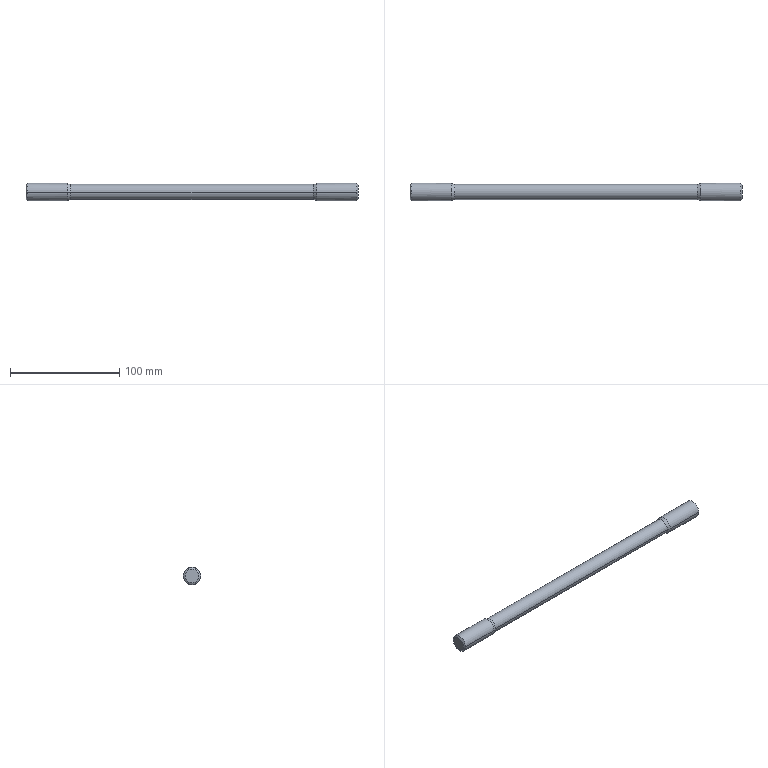Part | SolidWorks | features MirrorPattern 2, LPattern 1, RevCut 1, Revolution 1 | 1 solid | 16 faces | box 304 x 16 x 16 mm | volume 49717 mm3 | cone 8 | cylinder 6 | plane 2 | commonest cylinder face diameters 16 x4 13.856 x2
STEP:
#1=CARTESIAN_POINT('',(152.,0.,-6.268));
#2=VERTEX_POINT('',#1);
#3=CARTESIAN_POINT('',(152.,0.,6.268));
#4=VERTEX_POINT('',#3);
#5=CARTESIAN_POINT('',(152.,0.,0.));
#6=DIRECTION('',(-1.,0.,0.));
#7=DIRECTION('',(0.,0.,1.));
#8=AXIS2_PLACEMENT_3D('',#5,#6,#7);
#9=CIRCLE('',#8,6.268);
#10=EDGE_CURVE('',#2,#4,#9,.T.);
#11=ORIENTED_EDGE('',*,*,#10,.T.);
#12=CARTESIAN_POINT('',(151.,0.,8.));
#13=VERTEX_POINT('',#12);
#14=CARTESIAN_POINT('',(152.,0.,6.268));
#15=DIRECTION('',(-0.5,0.,0.866));
#16=VECTOR('',#15,1000.);
#17=LINE('',#14,#16);
#18=EDGE_CURVE('',#4,#13,#17,.T.);
#19=ORIENTED_EDGE('',*,*,#18,.T.);
#20=CARTESIAN_POINT('',(151.,-8.,0.));
#21=VERTEX_POINT('',#20);
#22=CARTESIAN_POINT('',(151.,0.,0.));
#23=DIRECTION('',(-1.,0.,0.));
#24=DIRECTION('',(0.,0.,1.));
#25=AXIS2_PLACEMENT_3D('',#22,#23,#24);
#26=CIRCLE('',#25,8.);
#27=EDGE_CURVE('',#21,#13,#26,.T.);
#28=ORIENTED_EDGE('',*,*,#27,.F.);
#29=CARTESIAN_POINT('',(151.,0.,-8.));
#30=VERTEX_POINT('',#29);
#31=CARTESIAN_POINT('',(151.,0.,0.));
#32=DIRECTION('',(-1.,0.,0.));
#33=DIRECTION('',(0.,0.,1.));
#34=AXIS2_PLACEMENT_3D('',#31,#32,#33);
#35=CIRCLE('',#34,8.);
#36=EDGE_CURVE('',#30,#21,#35,.T.);
#37=ORIENTED_EDGE('',*,*,#36,.F.);
#38=CARTESIAN_POINT('',(152.,0.,-6.268));
#39=DIRECTION('',(-0.5,0.,-0.866));
#40=VECTOR('',#39,1000.);
#41=LINE('',#38,#40);
#42=EDGE_CURVE('',#2,#30,#41,.T.);
#43=ORIENTED_EDGE('',*,*,#42,.F.);
#44=EDGE_LOOP('',(#11,#19,#28,#37,#43));
#45=FACE_OUTER_BOUND('',#44,.T.);
#46=CARTESIAN_POINT('',(152.,0.,0.));
#47=DIRECTION('',(-1.,0.,0.));
#48=DIRECTION('',(0.,0.,-1.));
#49=AXIS2_PLACEMENT_3D('',#46,#47,#48);
#50=CONICAL_SURFACE('',#49,6.268,1.047);
#51=ADVANCED_FACE('',(#45),#50,.T.);
#52=CARTESIAN_POINT('',(-152.,0.,6.268));
#53=VERTEX_POINT('',#52);
#54=CARTESIAN_POINT('',(-152.,0.,-6.268));
#55=VERTEX_POINT('',#54);
#56=CARTESIAN_POINT('',(-152.,0.,0.));
#57=DIRECTION('',(-1.,0.,0.));
#58=DIRECTION('',(0.,0.,1.));
#59=AXIS2_PLACEMENT_3D('',#56,#57,#58);
#60=CIRCLE('',#59,6.268);
#61=EDGE_CURVE('',#53,#55,#60,.T.);
#62=ORIENTED_EDGE('',*,*,#61,.F.);
#63=CARTESIAN_POINT('',(-151.,0.,8.));
#64=VERTEX_POINT('',#63);
#65=CARTESIAN_POINT('',(-152.,0.,6.268));
#66=DIRECTION('',(0.5,0.,0.866));
#67=VECTOR('',#66,1000.);
#68=LINE('',#65,#67);
#69=EDGE_CURVE('',#53,#64,#68,.T.);
#70=ORIENTED_EDGE('',*,*,#69,.T.);
#71=CARTESIAN_POINT('',(-151.,8.,0.));
#72=VERTEX_POINT('',#71);
#73=CARTESIAN_POINT('',(-151.,0.,0.));
#74=DIRECTION('',(-1.,0.,0.));
#75=DIRECTION('',(0.,0.,1.));
#76=AXIS2_PLACEMENT_3D('',#73,#74,#75);
#77=CIRCLE('',#76,8.);
#78=EDGE_CURVE('',#64,#72,#77,.T.);
#79=ORIENTED_EDGE('',*,*,#78,.T.);
#80=CARTESIAN_POINT('',(-151.,0.,-8.));
#81=VERTEX_POINT('',#80);
#82=CARTESIAN_POINT('',(-151.,0.,0.));
#83=DIRECTION('',(-1.,0.,0.));
#84=DIRECTION('',(0.,0.,1.));
#85=AXIS2_PLACEMENT_3D('',#82,#83,#84);
#86=CIRCLE('',#85,8.);
#87=EDGE_CURVE('',#72,#81,#86,.T.);
#88=ORIENTED_EDGE('',*,*,#87,.T.);
#89=CARTESIAN_POINT('',(-152.,0.,-6.268));
#90=DIRECTION('',(0.5,0.,-0.866));
#91=VECTOR('',#90,1000.);
#92=LINE('',#89,#91);
#93=EDGE_CURVE('',#55,#81,#92,.T.);
#94=ORIENTED_EDGE('',*,*,#93,.F.);
#95=EDGE_LOOP('',(#62,#70,#79,#88,#94));
#96=FACE_OUTER_BOUND('',#95,.T.);
#97=CARTESIAN_POINT('',(-152.,0.,0.));
#98=DIRECTION('',(1.,0.,0.));
#99=DIRECTION('',(0.,0.,-1.));
#100=AXIS2_PLACEMENT_3D('',#97,#98,#99);
#101=CONICAL_SURFACE('',#100,6.268,1.047);
#102=ADVANCED_FACE('',(#96),#101,.T.);
#103=CARTESIAN_POINT('',(-111.2,-6.928,0.));
#104=VERTEX_POINT('',#103);
#105=CARTESIAN_POINT('',(-111.2,6.928,0.));
#106=VERTEX_POINT('',#105);
#107=CARTESIAN_POINT('',(-111.2,0.,0.));
#108=DIRECTION('',(-1.,0.,0.));
#109=DIRECTION('',(0.,-1.,0.));
#110=AXIS2_PLACEMENT_3D('',#107,#108,#109);
#111=CIRCLE('',#110,6.928);
#112=EDGE_CURVE('',#104,#106,#111,.T.);
#113=ORIENTED_EDGE('',*,*,#112,.T.);
#114=CARTESIAN_POINT('',(-114.,8.,0.));
#115=VERTEX_POINT('',#114);
#116=CARTESIAN_POINT('',(-111.2,6.928,0.));
#117=DIRECTION('',(-0.9339,0.3575,0.));
#118=VECTOR('',#117,1000.);
#119=LINE('',#116,#118);
#120=EDGE_CURVE('',#106,#115,#119,.T.);
#121=ORIENTED_EDGE('',*,*,#120,.T.);
#122=CARTESIAN_POINT('',(-114.,-8.,0.));
#123=VERTEX_POINT('',#122);
#124=CARTESIAN_POINT('',(-114.,0.,0.));
#125=DIRECTION('',(-1.,0.,0.));
#126=DIRECTION('',(0.,-1.,0.));
#127=AXIS2_PLACEMENT_3D('',#124,#125,#126);
#128=CIRCLE('',#127,8.);
#129=EDGE_CURVE('',#123,#115,#128,.T.);
#130=ORIENTED_EDGE('',*,*,#129,.F.);
#131=CARTESIAN_POINT('',(-111.2,-6.928,0.));
#132=DIRECTION('',(-0.9339,-0.3575,0.));
#133=VECTOR('',#132,1000.);
#134=LINE('',#131,#133);
#135=EDGE_CURVE('',#104,#123,#134,.T.);
#136=ORIENTED_EDGE('',*,*,#135,.F.);
#137=EDGE_LOOP('',(#113,#121,#130,#136));
#138=FACE_OUTER_BOUND('',#137,.T.);
#139=CARTESIAN_POINT('',(-111.2,0.,0.));
#140=DIRECTION('',(-1.,0.,0.));
#141=DIRECTION('',(0.,-1.,0.));
#142=AXIS2_PLACEMENT_3D('',#139,#140,#141);
#143=CONICAL_SURFACE('',#142,6.928,0.3656);
#144=ADVANCED_FACE('',(#138),#143,.T.);
#145=CARTESIAN_POINT('',(111.2,-6.928,0.));
#146=VERTEX_POINT('',#145);
#147=CARTESIAN_POINT('',(111.2,6.928,0.));
#148=VERTEX_POINT('',#147);
#149=CARTESIAN_POINT('',(111.2,0.,0.));
#150=DIRECTION('',(-1.,0.,0.));
#151=DIRECTION('',(0.,-1.,0.));
#152=AXIS2_PLACEMENT_3D('',#149,#150,#151);
#153=CIRCLE('',#152,6.928);
#154=EDGE_CURVE('',#146,#148,#153,.T.);
#155=ORIENTED_EDGE('',*,*,#154,.T.);
#156=CARTESIAN_POINT('',(-152.,6.928,0.));
#157=DIRECTION('',(-1.,0.,0.));
#158=VECTOR('',#157,1000.);
#159=LINE('',#156,#158);
#160=EDGE_CURVE('',#148,#106,#159,.T.);
#161=ORIENTED_EDGE('',*,*,#160,.T.);
#162=ORIENTED_EDGE('',*,*,#112,.F.);
#163=CARTESIAN_POINT('',(-152.,-6.928,0.));
#164=DIRECTION('',(-1.,0.,0.));
#165=VECTOR('',#164,1000.);
#166=LINE('',#163,#165);
#167=EDGE_CURVE('',#146,#104,#166,.T.);
#168=ORIENTED_EDGE('',*,*,#167,.F.);
#169=EDGE_LOOP('',(#155,#161,#162,#168));
#170=FACE_OUTER_BOUND('',#169,.T.);
#171=CARTESIAN_POINT('',(-152.,0.,0.));
#172=DIRECTION('',(-1.,0.,0.));
#173=DIRECTION('',(0.,-1.,0.));
#174=AXIS2_PLACEMENT_3D('',#171,#172,#173);
#175=CYLINDRICAL_SURFACE('',#174,6.928);
#176=ADVANCED_FACE('',(#170),#175,.T.);
#177=ORIENTED_EDGE('',*,*,#154,.F.);
#178=CARTESIAN_POINT('',(114.,-8.,0.));
#179=VERTEX_POINT('',#178);
#180=CARTESIAN_POINT('',(114.,-8.,0.));
#181=DIRECTION('',(0.9339,-0.3575,0.));
#182=VECTOR('',#181,1000.);
#183=LINE('',#180,#182);
#184=EDGE_CURVE('',#146,#179,#183,.T.);
#185=ORIENTED_EDGE('',*,*,#184,.T.);
#186=CARTESIAN_POINT('',(114.,8.,0.));
#187=VERTEX_POINT('',#186);
#188=CARTESIAN_POINT('',(114.,0.,0.));
#189=DIRECTION('',(-1.,0.,0.));
#190=DIRECTION('',(0.,-1.,0.));
#191=AXIS2_PLACEMENT_3D('',#188,#189,#190);
#192=CIRCLE('',#191,8.);
#193=EDGE_CURVE('',#179,#187,#192,.T.);
#194=ORIENTED_EDGE('',*,*,#193,.T.);
#195=CARTESIAN_POINT('',(114.,8.,0.));
#196=DIRECTION('',(0.9339,0.3575,0.));
#197=VECTOR('',#196,1000.);
#198=LINE('',#195,#197);
#199=EDGE_CURVE('',#148,#187,#198,.T.);
#200=ORIENTED_EDGE('',*,*,#199,.F.);
#201=EDGE_LOOP('',(#177,#185,#194,#200));
#202=FACE_OUTER_BOUND('',#201,.T.);
#203=CARTESIAN_POINT('',(114.,0.,0.));
#204=DIRECTION('',(1.,0.,0.));
#205=DIRECTION('',(0.,1.,0.));
#206=AXIS2_PLACEMENT_3D('',#203,#204,#205);
#207=CONICAL_SURFACE('',#206,8.,0.3656);
#208=ADVANCED_FACE('',(#202),#207,.T.);
#209=ORIENTED_EDGE('',*,*,#129,.T.);
#210=CARTESIAN_POINT('',(-152.,8.,0.));
#211=DIRECTION('',(-1.,0.,0.));
#212=VECTOR('',#211,1000.);
#213=LINE('',#210,#212);
#214=EDGE_CURVE('',#115,#72,#213,.T.);
#215=ORIENTED_EDGE('',*,*,#214,.T.);
#216=ORIENTED_EDGE('',*,*,#78,.F.);
#217=CARTESIAN_POINT('',(-151.,-8.,0.));
#218=VERTEX_POINT('',#217);
#219=CARTESIAN_POINT('',(-151.,0.,0.));
#220=DIRECTION('',(-1.,0.,0.));
#221=DIRECTION('',(0.,0.,1.));
#222=AXIS2_PLACEMENT_3D('',#219,#220,#221);
#223=CIRCLE('',#222,8.);
#224=EDGE_CURVE('',#218,#64,#223,.T.);
#225=ORIENTED_EDGE('',*,*,#224,.F.);
#226=CARTESIAN_POINT('',(-152.,-8.,0.));
#227=DIRECTION('',(-1.,0.,0.));
#228=VECTOR('',#227,1000.);
#229=LINE('',#226,#228);
#230=EDGE_CURVE('',#123,#218,#229,.T.);
#231=ORIENTED_EDGE('',*,*,#230,.F.);
#232=EDGE_LOOP('',(#209,#215,#216,#225,#231));
#233=FACE_OUTER_BOUND('',#232,.T.);
#234=CARTESIAN_POINT('',(-152.,0.,0.));
#235=DIRECTION('',(-1.,0.,0.));
#236=DIRECTION('',(0.,-1.,0.));
#237=AXIS2_PLACEMENT_3D('',#234,#235,#236);
#238=CYLINDRICAL_SURFACE('',#237,8.);
#239=ADVANCED_FACE('',(#233),#238,.T.);
#240=ORIENTED_EDGE('',*,*,#27,.T.);
#241=CARTESIAN_POINT('',(151.,8.,0.));
#242=VERTEX_POINT('',#241);
#243=CARTESIAN_POINT('',(151.,0.,0.));
#244=DIRECTION('',(-1.,0.,0.));
#245=DIRECTION('',(0.,0.,1.));
#246=AXIS2_PLACEMENT_3D('',#243,#244,#245);
#247=CIRCLE('',#246,8.);
#248=EDGE_CURVE('',#13,#242,#247,.T.);
#249=ORIENTED_EDGE('',*,*,#248,.T.);
#250=CARTESIAN_POINT('',(-152.,8.,0.));
#251=DIRECTION('',(-1.,0.,0.));
#252=VECTOR('',#251,1000.);
#253=LINE('',#250,#252);
#254=EDGE_CURVE('',#242,#187,#253,.T.);
#255=ORIENTED_EDGE('',*,*,#254,.T.);
#256=ORIENTED_EDGE('',*,*,#193,.F.);
#257=CARTESIAN_POINT('',(-152.,-8.,0.));
#258=DIRECTION('',(-1.,0.,0.));
#259=VECTOR('',#258,1000.);
#260=LINE('',#257,#259);
#261=EDGE_CURVE('',#21,#179,#260,.T.);
#262=ORIENTED_EDGE('',*,*,#261,.F.);
#263=EDGE_LOOP('',(#240,#249,#255,#256,#262));
#264=FACE_OUTER_BOUND('',#263,.T.);
#265=CARTESIAN_POINT('',(-152.,0.,0.));
#266=DIRECTION('',(-1.,0.,0.));
#267=DIRECTION('',(0.,-1.,0.));
#268=AXIS2_PLACEMENT_3D('',#265,#266,#267);
#269=CYLINDRICAL_SURFACE('',#268,8.);
#270=ADVANCED_FACE('',(#264),#269,.T.);
#271=ORIENTED_EDGE('',*,*,#254,.F.);
#272=CARTESIAN_POINT('',(151.,0.,0.));
#273=DIRECTION('',(-1.,0.,0.));
#274=DIRECTION('',(0.,0.,1.));
#275=AXIS2_PLACEMENT_3D('',#272,#273,#274);
#276=CIRCLE('',#275,8.);
#277=EDGE_CURVE('',#242,#30,#276,.T.);
#278=ORIENTED_EDGE('',*,*,#277,.T.);
#279=ORIENTED_EDGE('',*,*,#36,.T.);
#280=ORIENTED_EDGE('',*,*,#261,.T.);
#281=CARTESIAN_POINT('',(114.,0.,0.));
#282=DIRECTION('',(-1.,0.,0.));
#283=DIRECTION('',(0.,-1.,0.));
#284=AXIS2_PLACEMENT_3D('',#281,#282,#283);
#285=CIRCLE('',#284,8.);
#286=EDGE_CURVE('',#187,#179,#285,.T.);
#287=ORIENTED_EDGE('',*,*,#286,.F.);
#288=EDGE_LOOP('',(#271,#278,#279,#280,#287));
#289=FACE_OUTER_BOUND('',#288,.T.);
#290=CARTESIAN_POINT('',(-152.,0.,0.));
#291=DIRECTION('',(-1.,0.,0.));
#292=DIRECTION('',(0.,-1.,0.));
#293=AXIS2_PLACEMENT_3D('',#290,#291,#292);
#294=CYLINDRICAL_SURFACE('',#293,8.);
#295=ADVANCED_FACE('',(#289),#294,.T.);
#296=ORIENTED_EDGE('',*,*,#214,.F.);
#297=CARTESIAN_POINT('',(-114.,0.,0.));
#298=DIRECTION('',(-1.,0.,0.));
#299=DIRECTION('',(0.,-1.,0.));
#300=AXIS2_PLACEMENT_3D('',#297,#298,#299);
#301=CIRCLE('',#300,8.);
#302=EDGE_CURVE('',#115,#123,#301,.T.);
#303=ORIENTED_EDGE('',*,*,#302,.T.);
#304=ORIENTED_EDGE('',*,*,#230,.T.);
#305=CARTESIAN_POINT('',(-151.,0.,0.));
#306=DIRECTION('',(-1.,0.,0.));
#307=DIRECTION('',(0.,0.,1.));
#308=AXIS2_PLACEMENT_3D('',#305,#306,#307);
#309=CIRCLE('',#308,8.);
#310=EDGE_CURVE('',#81,#218,#309,.T.);
#311=ORIENTED_EDGE('',*,*,#310,.F.);
#312=ORIENTED_EDGE('',*,*,#87,.F.);
#313=EDGE_LOOP('',(#296,#303,#304,#311,#312));
#314=FACE_OUTER_BOUND('',#313,.T.);
#315=CARTESIAN_POINT('',(-152.,0.,0.));
#316=DIRECTION('',(-1.,0.,0.));
#317=DIRECTION('',(0.,-1.,0.));
#318=AXIS2_PLACEMENT_3D('',#315,#316,#317);
#319=CYLINDRICAL_SURFACE('',#318,8.);
#320=ADVANCED_FACE('',(#314),#319,.T.);
#321=ORIENTED_EDGE('',*,*,#184,.F.);
#322=CARTESIAN_POINT('',(111.2,0.,0.));
#323=DIRECTION('',(-1.,0.,0.));
#324=DIRECTION('',(0.,-1.,0.));
#325=AXIS2_PLACEMENT_3D('',#322,#323,#324);
#326=CIRCLE('',#325,6.928);
#327=EDGE_CURVE('',#148,#146,#326,.T.);
#328=ORIENTED_EDGE('',*,*,#327,.F.);
#329=ORIENTED_EDGE('',*,*,#199,.T.);
#330=ORIENTED_EDGE('',*,*,#286,.T.);
#331=EDGE_LOOP('',(#321,#328,#329,#330));
#332=FACE_OUTER_BOUND('',#331,.T.);
#333=CARTESIAN_POINT('',(114.,0.,0.));
#334=DIRECTION('',(1.,0.,0.));
#335=DIRECTION('',(0.,1.,0.));
#336=AXIS2_PLACEMENT_3D('',#333,#334,#335);
#337=CONICAL_SURFACE('',#336,8.,0.3656);
#338=ADVANCED_FACE('',(#332),#337,.T.);
#339=ORIENTED_EDGE('',*,*,#160,.F.);
#340=ORIENTED_EDGE('',*,*,#327,.T.);
#341=ORIENTED_EDGE('',*,*,#167,.T.);
#342=CARTESIAN_POINT('',(-111.2,0.,0.));
#343=DIRECTION('',(-1.,0.,0.));
#344=DIRECTION('',(0.,-1.,0.));
#345=AXIS2_PLACEMENT_3D('',#342,#343,#344);
#346=CIRCLE('',#345,6.928);
#347=EDGE_CURVE('',#106,#104,#346,.T.);
#348=ORIENTED_EDGE('',*,*,#347,.F.);
#349=EDGE_LOOP('',(#339,#340,#341,#348));
#350=FACE_OUTER_BOUND('',#349,.T.);
#351=CARTESIAN_POINT('',(-152.,0.,0.));
#352=DIRECTION('',(-1.,0.,0.));
#353=DIRECTION('',(0.,-1.,0.));
#354=AXIS2_PLACEMENT_3D('',#351,#352,#353);
#355=CYLINDRICAL_SURFACE('',#354,6.928);
#356=ADVANCED_FACE('',(#350),#355,.T.);
#357=ORIENTED_EDGE('',*,*,#120,.F.);
#358=ORIENTED_EDGE('',*,*,#347,.T.);
#359=ORIENTED_EDGE('',*,*,#135,.T.);
#360=ORIENTED_EDGE('',*,*,#302,.F.);
#361=EDGE_LOOP('',(#357,#358,#359,#360));
#362=FACE_OUTER_BOUND('',#361,.T.);
#363=CARTESIAN_POINT('',(-111.2,0.,0.));
#364=DIRECTION('',(-1.,0.,0.));
#365=DIRECTION('',(0.,-1.,0.));
#366=AXIS2_PLACEMENT_3D('',#363,#364,#365);
#367=CONICAL_SURFACE('',#366,6.928,0.3656);
#368=ADVANCED_FACE('',(#362),#367,.T.);
#369=ORIENTED_EDGE('',*,*,#69,.F.);
#370=CARTESIAN_POINT('',(-152.,0.,0.));
#371=DIRECTION('',(-1.,0.,0.));
#372=DIRECTION('',(0.,0.,1.));
#373=AXIS2_PLACEMENT_3D('',#370,#371,#372);
#374=CIRCLE('',#373,6.268);
#375=EDGE_CURVE('',#55,#53,#374,.T.);
#376=ORIENTED_EDGE('',*,*,#375,.F.);
#377=ORIENTED_EDGE('',*,*,#93,.T.);
#378=ORIENTED_EDGE('',*,*,#310,.T.);
#379=ORIENTED_EDGE('',*,*,#224,.T.);
#380=EDGE_LOOP('',(#369,#376,#377,#378,#379));
#381=FACE_OUTER_BOUND('',#380,.T.);
#382=CARTESIAN_POINT('',(-152.,0.,0.));
#383=DIRECTION('',(1.,0.,0.));
#384=DIRECTION('',(0.,0.,-1.));
#385=AXIS2_PLACEMENT_3D('',#382,#383,#384);
#386=CONICAL_SURFACE('',#385,6.268,1.047);
#387=ADVANCED_FACE('',(#381),#386,.T.);
#388=ORIENTED_EDGE('',*,*,#375,.T.);
#389=ORIENTED_EDGE('',*,*,#61,.T.);
#390=EDGE_LOOP('',(#388,#389));
#391=FACE_OUTER_BOUND('',#390,.T.);
#392=CARTESIAN_POINT('',(-152.,8.,0.));
#393=DIRECTION('',(1.,0.,0.));
#394=DIRECTION('',(0.,1.,0.));
#395=AXIS2_PLACEMENT_3D('',#392,#393,#394);
#396=PLANE('',#395);
#397=ADVANCED_FACE('',(#391),#396,.F.);
#398=ORIENTED_EDGE('',*,*,#18,.F.);
#399=CARTESIAN_POINT('',(152.,0.,0.));
#400=DIRECTION('',(-1.,0.,0.));
#401=DIRECTION('',(0.,0.,1.));
#402=AXIS2_PLACEMENT_3D('',#399,#400,#401);
#403=CIRCLE('',#402,6.268);
#404=EDGE_CURVE('',#4,#2,#403,.T.);
#405=ORIENTED_EDGE('',*,*,#404,.T.);
#406=ORIENTED_EDGE('',*,*,#42,.T.);
#407=ORIENTED_EDGE('',*,*,#277,.F.);
#408=ORIENTED_EDGE('',*,*,#248,.F.);
#409=EDGE_LOOP('',(#398,#405,#406,#407,#408));
#410=FACE_OUTER_BOUND('',#409,.T.);
#411=CARTESIAN_POINT('',(152.,0.,0.));
#412=DIRECTION('',(-1.,0.,0.));
#413=DIRECTION('',(0.,0.,-1.));
#414=AXIS2_PLACEMENT_3D('',#411,#412,#413);
#415=CONICAL_SURFACE('',#414,6.268,1.047);
#416=ADVANCED_FACE('',(#410),#415,.T.);
#417=ORIENTED_EDGE('',*,*,#10,.F.);
#418=ORIENTED_EDGE('',*,*,#404,.F.);
#419=EDGE_LOOP('',(#417,#418));
#420=FACE_OUTER_BOUND('',#419,.T.);
#421=CARTESIAN_POINT('',(152.,8.,0.));
#422=DIRECTION('',(-1.,0.,0.));
#423=DIRECTION('',(0.,-1.,0.));
#424=AXIS2_PLACEMENT_3D('',#421,#422,#423);
#425=PLANE('',#424);
#426=ADVANCED_FACE('',(#420),#425,.F.);
#427=CLOSED_SHELL('',(#51,#102,#144,#176,#208,#239,#270,#295,#320,#338,#356,#368,#387,#397,#416,#426));
#428=MANIFOLD_SOLID_BREP('',#427);
#429=CARTESIAN_POINT('',(0.,0.,0.));
#430=DIRECTION('',(0.,0.,1.));
#431=DIRECTION('',(1.,0.,0.));
#432=AXIS2_PLACEMENT_3D('',#429,#430,#431);
#433=(LENGTH_UNIT()NAMED_UNIT(*)SI_UNIT(.MILLI.,.METRE.));
#434=UNCERTAINTY_MEASURE_WITH_UNIT(LENGTH_MEASURE(0.00001),#433,'','');
#435=(NAMED_UNIT(*)PLANE_ANGLE_UNIT()SI_UNIT($,.RADIAN.));
#436=(NAMED_UNIT(*)SI_UNIT($,.STERADIAN.)SOLID_ANGLE_UNIT());
#437=(GEOMETRIC_REPRESENTATION_CONTEXT(3)GLOBAL_UNCERTAINTY_ASSIGNED_CONTEXT((#434))GLOBAL_UNIT_ASSIGNED_CONTEXT((#433,#435,#436))REPRESENTATION_CONTEXT('',''));
#438=ADVANCED_BREP_SHAPE_REPRESENTATION('',(#428,#432),#437);